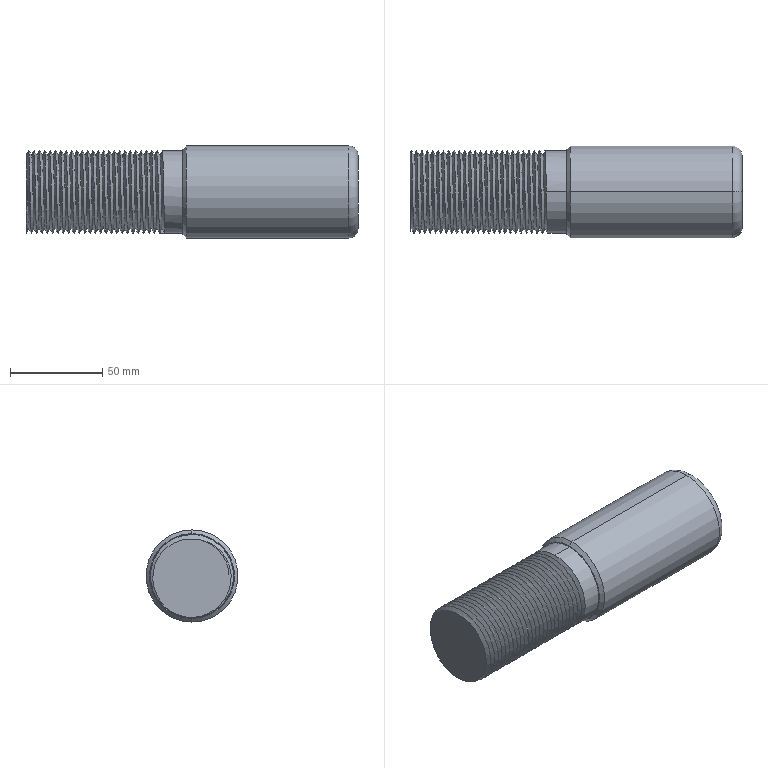Part | SolidWorks | 1 solid | 16 faces | box 180.002 x 50 x 50 mm | volume 309551 mm3 | plane 5 | cylinder 5 | torus 2 | cone 2 | spline 2 | commonest cylinder face diameters 45 x3 50 x2